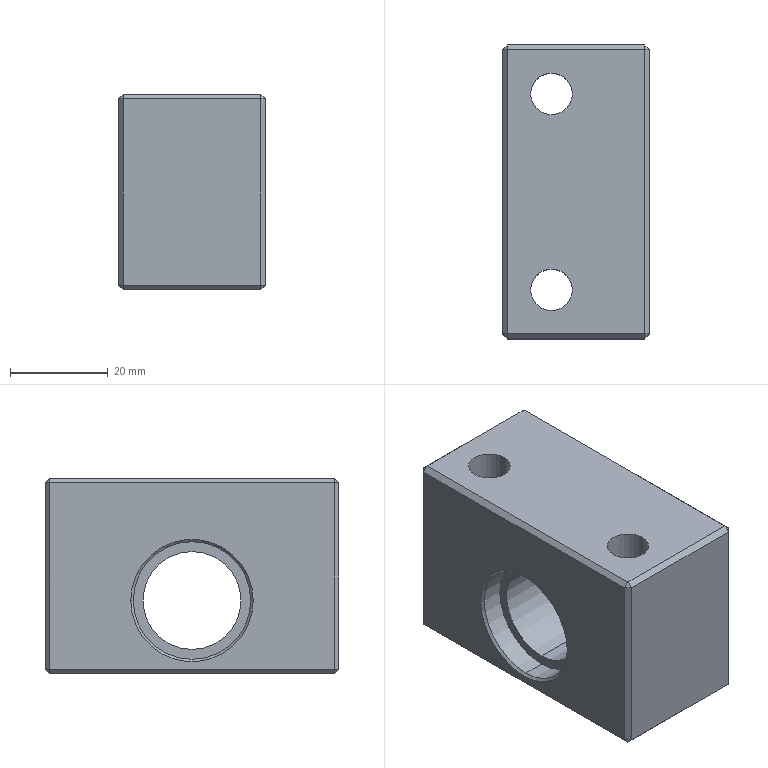Part | STEP file | Feed swing arm fixing piece | 1 solid | 52 faces | box 30 x 60 x 40 mm | volume 54813 mm3 | plane 30 | cylinder 14 | cone 8 | commonest cylinder face diameters 8.5 x4 14 x4 24 x4 20 x2